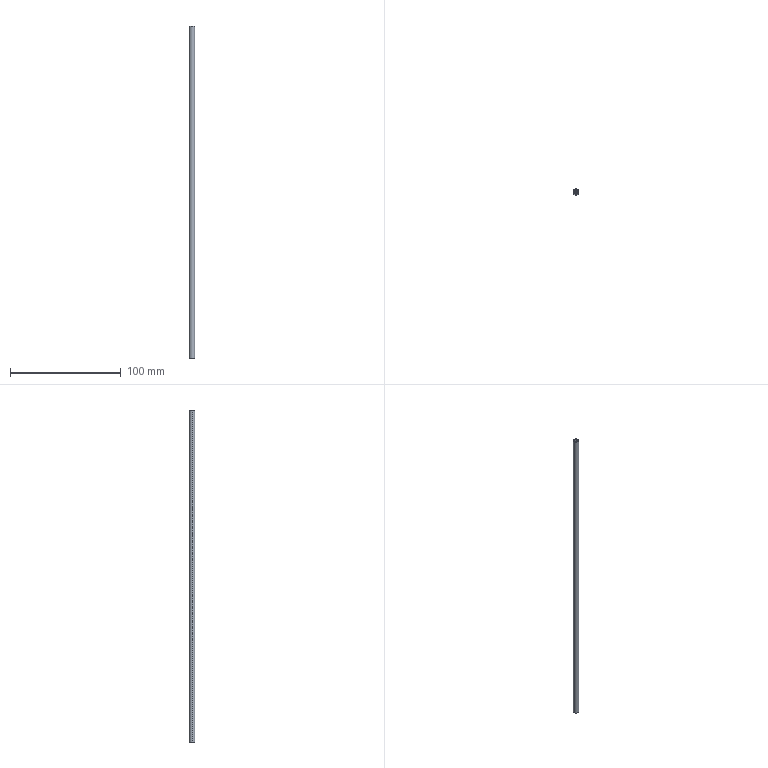Part | SolidWorks | features Extrusion 1 | 1 solid | 6 faces | box 5 x 5 x 300 mm | volume 4418 mm3 | cylinder 4 | plane 2 | commonest cylinder face diameters 2.5 x2 5 x2
STEP:
#1=CARTESIAN_POINT('',(-1.25,0.,300.));
#2=VERTEX_POINT('',#1);
#3=CARTESIAN_POINT('',(1.25,0.,300.));
#4=VERTEX_POINT('',#3);
#5=CARTESIAN_POINT('',(0.,0.,300.));
#6=DIRECTION('',(0.,0.,1.));
#7=DIRECTION('',(1.,0.,0.));
#8=AXIS2_PLACEMENT_3D('',#5,#6,#7);
#9=CIRCLE('',#8,1.25);
#10=EDGE_CURVE('',#2,#4,#9,.T.);
#11=ORIENTED_EDGE('',*,*,#10,.T.);
#12=CARTESIAN_POINT('',(1.25,0.,0.));
#13=VERTEX_POINT('',#12);
#14=CARTESIAN_POINT('',(1.25,0.,300.));
#15=DIRECTION('',(0.,0.,-1.));
#16=VECTOR('',#15,1000.);
#17=LINE('',#14,#16);
#18=EDGE_CURVE('',#4,#13,#17,.T.);
#19=ORIENTED_EDGE('',*,*,#18,.T.);
#20=CARTESIAN_POINT('',(-1.25,0.,0.));
#21=VERTEX_POINT('',#20);
#22=CARTESIAN_POINT('',(0.,0.,0.));
#23=DIRECTION('',(0.,0.,1.));
#24=DIRECTION('',(1.,0.,0.));
#25=AXIS2_PLACEMENT_3D('',#22,#23,#24);
#26=CIRCLE('',#25,1.25);
#27=EDGE_CURVE('',#21,#13,#26,.T.);
#28=ORIENTED_EDGE('',*,*,#27,.F.);
#29=CARTESIAN_POINT('',(-1.25,0.,300.));
#30=DIRECTION('',(0.,0.,-1.));
#31=VECTOR('',#30,1000.);
#32=LINE('',#29,#31);
#33=EDGE_CURVE('',#2,#21,#32,.T.);
#34=ORIENTED_EDGE('',*,*,#33,.F.);
#35=EDGE_LOOP('',(#11,#19,#28,#34));
#36=FACE_OUTER_BOUND('',#35,.T.);
#37=CARTESIAN_POINT('',(0.,0.,300.));
#38=DIRECTION('',(0.,0.,-1.));
#39=DIRECTION('',(-1.,0.,0.));
#40=AXIS2_PLACEMENT_3D('',#37,#38,#39);
#41=CYLINDRICAL_SURFACE('',#40,1.25);
#42=ADVANCED_FACE('',(#36),#41,.F.);
#43=CARTESIAN_POINT('',(2.5,0.,300.));
#44=VERTEX_POINT('',#43);
#45=CARTESIAN_POINT('',(-2.5,0.,300.));
#46=VERTEX_POINT('',#45);
#47=CARTESIAN_POINT('',(0.,0.,300.));
#48=DIRECTION('',(0.,0.,1.));
#49=DIRECTION('',(1.,0.,0.));
#50=AXIS2_PLACEMENT_3D('',#47,#48,#49);
#51=CIRCLE('',#50,2.5);
#52=EDGE_CURVE('',#44,#46,#51,.T.);
#53=ORIENTED_EDGE('',*,*,#52,.F.);
#54=CARTESIAN_POINT('',(2.5,0.,0.));
#55=VERTEX_POINT('',#54);
#56=CARTESIAN_POINT('',(2.5,0.,300.));
#57=DIRECTION('',(0.,0.,-1.));
#58=VECTOR('',#57,1000.);
#59=LINE('',#56,#58);
#60=EDGE_CURVE('',#44,#55,#59,.T.);
#61=ORIENTED_EDGE('',*,*,#60,.T.);
#62=CARTESIAN_POINT('',(-2.5,0.,0.));
#63=VERTEX_POINT('',#62);
#64=CARTESIAN_POINT('',(0.,0.,0.));
#65=DIRECTION('',(0.,0.,1.));
#66=DIRECTION('',(1.,0.,0.));
#67=AXIS2_PLACEMENT_3D('',#64,#65,#66);
#68=CIRCLE('',#67,2.5);
#69=EDGE_CURVE('',#55,#63,#68,.T.);
#70=ORIENTED_EDGE('',*,*,#69,.T.);
#71=CARTESIAN_POINT('',(-2.5,0.,300.));
#72=DIRECTION('',(0.,0.,-1.));
#73=VECTOR('',#72,1000.);
#74=LINE('',#71,#73);
#75=EDGE_CURVE('',#46,#63,#74,.T.);
#76=ORIENTED_EDGE('',*,*,#75,.F.);
#77=EDGE_LOOP('',(#53,#61,#70,#76));
#78=FACE_OUTER_BOUND('',#77,.T.);
#79=CARTESIAN_POINT('',(0.,0.,300.));
#80=DIRECTION('',(0.,0.,-1.));
#81=DIRECTION('',(-1.,0.,0.));
#82=AXIS2_PLACEMENT_3D('',#79,#80,#81);
#83=CYLINDRICAL_SURFACE('',#82,2.5);
#84=ADVANCED_FACE('',(#78),#83,.T.);
#85=CARTESIAN_POINT('',(0.,0.,300.));
#86=DIRECTION('',(0.,0.,1.));
#87=DIRECTION('',(1.,0.,0.));
#88=AXIS2_PLACEMENT_3D('',#85,#86,#87);
#89=CIRCLE('',#88,2.5);
#90=EDGE_CURVE('',#46,#44,#89,.T.);
#91=ORIENTED_EDGE('',*,*,#90,.T.);
#92=ORIENTED_EDGE('',*,*,#52,.T.);
#93=EDGE_LOOP('',(#91,#92));
#94=FACE_OUTER_BOUND('',#93,.T.);
#95=ORIENTED_EDGE('',*,*,#10,.F.);
#96=CARTESIAN_POINT('',(0.,0.,300.));
#97=DIRECTION('',(0.,0.,1.));
#98=DIRECTION('',(1.,0.,0.));
#99=AXIS2_PLACEMENT_3D('',#96,#97,#98);
#100=CIRCLE('',#99,1.25);
#101=EDGE_CURVE('',#4,#2,#100,.T.);
#102=ORIENTED_EDGE('',*,*,#101,.F.);
#103=EDGE_LOOP('',(#95,#102));
#104=FACE_BOUND('',#103,.T.);
#105=CARTESIAN_POINT('',(0.,0.,300.));
#106=DIRECTION('',(0.,0.,1.));
#107=DIRECTION('',(1.,0.,0.));
#108=AXIS2_PLACEMENT_3D('',#105,#106,#107);
#109=PLANE('',#108);
#110=ADVANCED_FACE('',(#94,#104),#109,.T.);
#111=CARTESIAN_POINT('',(0.,0.,0.));
#112=DIRECTION('',(0.,0.,1.));
#113=DIRECTION('',(1.,0.,0.));
#114=AXIS2_PLACEMENT_3D('',#111,#112,#113);
#115=CIRCLE('',#114,2.5);
#116=EDGE_CURVE('',#63,#55,#115,.T.);
#117=ORIENTED_EDGE('',*,*,#116,.F.);
#118=ORIENTED_EDGE('',*,*,#69,.F.);
#119=EDGE_LOOP('',(#117,#118));
#120=FACE_OUTER_BOUND('',#119,.T.);
#121=ORIENTED_EDGE('',*,*,#27,.T.);
#122=CARTESIAN_POINT('',(0.,0.,0.));
#123=DIRECTION('',(0.,0.,1.));
#124=DIRECTION('',(1.,0.,0.));
#125=AXIS2_PLACEMENT_3D('',#122,#123,#124);
#126=CIRCLE('',#125,1.25);
#127=EDGE_CURVE('',#13,#21,#126,.T.);
#128=ORIENTED_EDGE('',*,*,#127,.T.);
#129=EDGE_LOOP('',(#121,#128));
#130=FACE_BOUND('',#129,.T.);
#131=CARTESIAN_POINT('',(0.,0.,0.));
#132=DIRECTION('',(0.,0.,1.));
#133=DIRECTION('',(1.,0.,0.));
#134=AXIS2_PLACEMENT_3D('',#131,#132,#133);
#135=PLANE('',#134);
#136=ADVANCED_FACE('',(#120,#130),#135,.F.);
#137=ORIENTED_EDGE('',*,*,#60,.F.);
#138=ORIENTED_EDGE('',*,*,#90,.F.);
#139=ORIENTED_EDGE('',*,*,#75,.T.);
#140=ORIENTED_EDGE('',*,*,#116,.T.);
#141=EDGE_LOOP('',(#137,#138,#139,#140));
#142=FACE_OUTER_BOUND('',#141,.T.);
#143=CARTESIAN_POINT('',(0.,0.,300.));
#144=DIRECTION('',(0.,0.,-1.));
#145=DIRECTION('',(-1.,0.,0.));
#146=AXIS2_PLACEMENT_3D('',#143,#144,#145);
#147=CYLINDRICAL_SURFACE('',#146,2.5);
#148=ADVANCED_FACE('',(#142),#147,.T.);
#149=ORIENTED_EDGE('',*,*,#18,.F.);
#150=ORIENTED_EDGE('',*,*,#101,.T.);
#151=ORIENTED_EDGE('',*,*,#33,.T.);
#152=ORIENTED_EDGE('',*,*,#127,.F.);
#153=EDGE_LOOP('',(#149,#150,#151,#152));
#154=FACE_OUTER_BOUND('',#153,.T.);
#155=CARTESIAN_POINT('',(0.,0.,300.));
#156=DIRECTION('',(0.,0.,-1.));
#157=DIRECTION('',(-1.,0.,0.));
#158=AXIS2_PLACEMENT_3D('',#155,#156,#157);
#159=CYLINDRICAL_SURFACE('',#158,1.25);
#160=ADVANCED_FACE('',(#154),#159,.F.);
#161=CLOSED_SHELL('',(#42,#84,#110,#136,#148,#160));
#162=MANIFOLD_SOLID_BREP('',#161);
#163=CARTESIAN_POINT('',(0.,0.,0.));
#164=DIRECTION('',(0.,0.,1.));
#165=DIRECTION('',(1.,0.,0.));
#166=AXIS2_PLACEMENT_3D('',#163,#164,#165);
#167=(LENGTH_UNIT()NAMED_UNIT(*)SI_UNIT(.MILLI.,.METRE.));
#168=UNCERTAINTY_MEASURE_WITH_UNIT(LENGTH_MEASURE(0.00001),#167,'','');
#169=(NAMED_UNIT(*)PLANE_ANGLE_UNIT()SI_UNIT($,.RADIAN.));
#170=(NAMED_UNIT(*)SI_UNIT($,.STERADIAN.)SOLID_ANGLE_UNIT());
#171=(GEOMETRIC_REPRESENTATION_CONTEXT(3)GLOBAL_UNCERTAINTY_ASSIGNED_CONTEXT((#168))GLOBAL_UNIT_ASSIGNED_CONTEXT((#167,#169,#170))REPRESENTATION_CONTEXT('',''));
#172=ADVANCED_BREP_SHAPE_REPRESENTATION('',(#162,#166),#171);